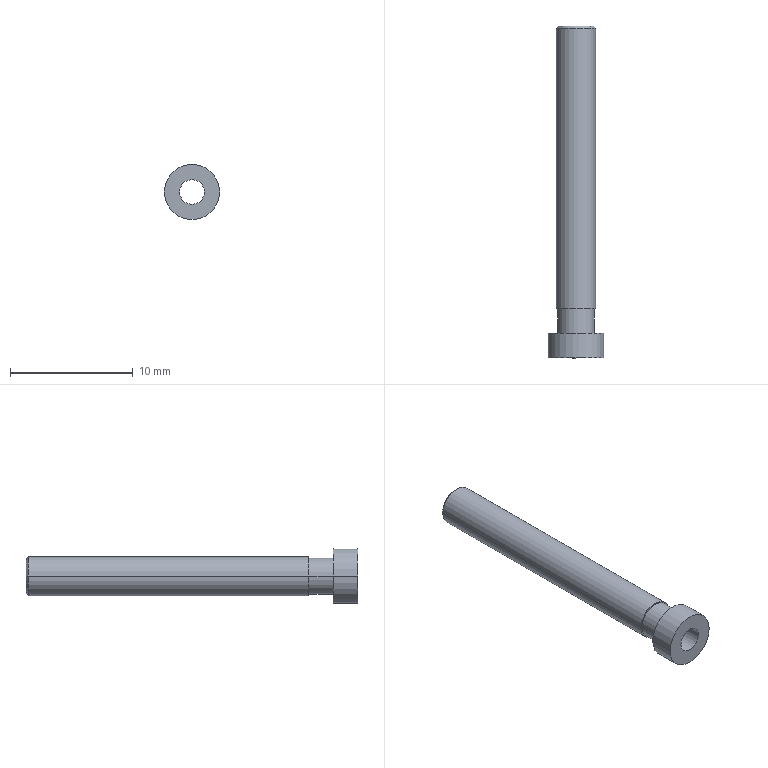Part | STEP file | BU-A08 | 1 solid | 14 faces | box 4.5 x 27 x 4.5 mm | volume 144.202 mm3 | cylinder 8 | plane 4 | cone 2 | commonest cylinder face diameters 2.02 x2 3 x2 3.2 x2 4.5 x2
STEP:
#1=CARTESIAN_POINT('',(0.,0.,0.));
#2=DIRECTION('',(0.,0.,1.));
#3=DIRECTION('',(1.,0.,0.));
#4=AXIS2_PLACEMENT_3D('',#1,#2,#3);
#5=CARTESIAN_POINT('',(-1.4,27.,0.));
#6=VERTEX_POINT('',#5);
#7=CARTESIAN_POINT('',(1.4,27.,0.));
#8=VERTEX_POINT('',#7);
#9=CARTESIAN_POINT('',(0.,27.,0.));
#10=DIRECTION('',(0.,1.,0.));
#11=DIRECTION('',(-1.,0.,0.));
#12=AXIS2_PLACEMENT_3D('',#9,#10,#11);
#13=CIRCLE('',#12,1.4);
#14=CARTESIAN_POINT('',(0.,26.8,0.));
#15=DIRECTION('',(0.,-1.,0.));
#16=DIRECTION('',(1.,0.,0.));
#17=AXIS2_PLACEMENT_3D('',#14,#15,#16);
#18=CONICAL_SURFACE('',#17,1.6,0.7854);
#19=CARTESIAN_POINT('',(3.142,-0.2));
#20=DIRECTION('',(-1.,0.));
#21=VECTOR('',#20,1.);
#22=LINE('',#19,#21);
#23=(GEOMETRIC_REPRESENTATION_CONTEXT(2)PARAMETRIC_REPRESENTATION_CONTEXT()REPRESENTATION_CONTEXT('',''));
#24=DEFINITIONAL_REPRESENTATION('',(#22),#23);
#25=PCURVE('',#18,#24);
#26=CARTESIAN_POINT('',(1.6,27.,0.));
#27=DIRECTION('',(0.,1.,0.));
#28=DIRECTION('',(-1.,0.,0.));
#29=AXIS2_PLACEMENT_3D('',#26,#27,#28);
#30=PLANE('',#29);
#31=CARTESIAN_POINT('',(1.6,0.));
#32=DIRECTION('',(1.,0.));
#33=AXIS2_PLACEMENT_2D('',#31,#32);
#34=CIRCLE('',#33,1.4);
#35=(GEOMETRIC_REPRESENTATION_CONTEXT(2)PARAMETRIC_REPRESENTATION_CONTEXT()REPRESENTATION_CONTEXT('',''));
#36=DEFINITIONAL_REPRESENTATION('',(#34),#35);
#37=PCURVE('',#30,#36);
#38=SURFACE_CURVE('',#13,(#25,#37),.PCURVE_S1.);
#39=EDGE_CURVE('',#6,#8,#38,.T.);
#40=ORIENTED_EDGE('',*,*,#39,.F.);
#41=CARTESIAN_POINT('',(-1.6,26.8,0.));
#42=VERTEX_POINT('',#41);
#43=CARTESIAN_POINT('',(-1.6,26.8,0.));
#44=DIRECTION('',(-0.7071,-0.7071,0.));
#45=VECTOR('',#44,1.);
#46=LINE('',#43,#45);
#47=CARTESIAN_POINT('',(3.142,0.));
#48=DIRECTION('',(0.,1.));
#49=VECTOR('',#48,1.);
#50=LINE('',#47,#49);
#51=(GEOMETRIC_REPRESENTATION_CONTEXT(2)PARAMETRIC_REPRESENTATION_CONTEXT()REPRESENTATION_CONTEXT('',''));
#52=DEFINITIONAL_REPRESENTATION('',(#50),#51);
#53=PCURVE('',#18,#52);
#54=CARTESIAN_POINT('',(0.,26.8,0.));
#55=DIRECTION('',(0.,-1.,0.));
#56=DIRECTION('',(1.,0.,0.));
#57=AXIS2_PLACEMENT_3D('',#54,#55,#56);
#58=CONICAL_SURFACE('',#57,1.6,0.7854);
#59=CARTESIAN_POINT('',(3.142,0.));
#60=DIRECTION('',(0.,1.));
#61=VECTOR('',#60,1.);
#62=LINE('',#59,#61);
#63=(GEOMETRIC_REPRESENTATION_CONTEXT(2)PARAMETRIC_REPRESENTATION_CONTEXT()REPRESENTATION_CONTEXT('',''));
#64=DEFINITIONAL_REPRESENTATION('',(#62),#63);
#65=PCURVE('',#58,#64);
#66=SURFACE_CURVE('',#46,(#53,#65),.PCURVE_S1.);
#67=EDGE_CURVE('',#6,#42,#66,.T.);
#68=ORIENTED_EDGE('',*,*,#67,.T.);
#69=CARTESIAN_POINT('',(1.6,26.8,0.));
#70=VERTEX_POINT('',#69);
#71=CARTESIAN_POINT('',(0.,26.8,0.));
#72=DIRECTION('',(0.,-1.,0.));
#73=DIRECTION('',(-1.,0.,0.));
#74=AXIS2_PLACEMENT_3D('',#71,#72,#73);
#75=CIRCLE('',#74,1.6);
#76=CARTESIAN_POINT('',(-3.142,0.));
#77=DIRECTION('',(1.,0.));
#78=VECTOR('',#77,1.);
#79=LINE('',#76,#78);
#80=(GEOMETRIC_REPRESENTATION_CONTEXT(2)PARAMETRIC_REPRESENTATION_CONTEXT()REPRESENTATION_CONTEXT('',''));
#81=DEFINITIONAL_REPRESENTATION('',(#79),#80);
#82=PCURVE('',#18,#81);
#83=CARTESIAN_POINT('',(0.,-1000.,0.));
#84=DIRECTION('',(0.,-1.,0.));
#85=DIRECTION('',(1.,0.,0.));
#86=AXIS2_PLACEMENT_3D('',#83,#84,#85);
#87=CYLINDRICAL_SURFACE('',#86,1.6);
#88=CARTESIAN_POINT('',(-3.142,-1026.8));
#89=DIRECTION('',(1.,0.));
#90=VECTOR('',#89,1.);
#91=LINE('',#88,#90);
#92=(GEOMETRIC_REPRESENTATION_CONTEXT(2)PARAMETRIC_REPRESENTATION_CONTEXT()REPRESENTATION_CONTEXT('',''));
#93=DEFINITIONAL_REPRESENTATION('',(#91),#92);
#94=PCURVE('',#87,#93);
#95=SURFACE_CURVE('',#75,(#82,#94),.PCURVE_S1.);
#96=EDGE_CURVE('',#70,#42,#95,.T.);
#97=ORIENTED_EDGE('',*,*,#96,.F.);
#98=CARTESIAN_POINT('',(1.6,26.8,0.));
#99=DIRECTION('',(0.7071,-0.7071,0.));
#100=VECTOR('',#99,1.);
#101=LINE('',#98,#100);
#102=CARTESIAN_POINT('',(0.,0.));
#103=DIRECTION('',(0.,1.));
#104=VECTOR('',#103,1.);
#105=LINE('',#102,#104);
#106=(GEOMETRIC_REPRESENTATION_CONTEXT(2)PARAMETRIC_REPRESENTATION_CONTEXT()REPRESENTATION_CONTEXT('',''));
#107=DEFINITIONAL_REPRESENTATION('',(#105),#106);
#108=PCURVE('',#18,#107);
#109=CARTESIAN_POINT('',(6.283,0.));
#110=DIRECTION('',(0.,1.));
#111=VECTOR('',#110,1.);
#112=LINE('',#109,#111);
#113=(GEOMETRIC_REPRESENTATION_CONTEXT(2)PARAMETRIC_REPRESENTATION_CONTEXT()REPRESENTATION_CONTEXT('',''));
#114=DEFINITIONAL_REPRESENTATION('',(#112),#113);
#115=PCURVE('',#58,#114);
#116=SURFACE_CURVE('',#101,(#108,#115),.PCURVE_S1.);
#117=EDGE_CURVE('',#8,#70,#116,.T.);
#118=ORIENTED_EDGE('',*,*,#117,.F.);
#119=EDGE_LOOP('',(#40,#68,#97,#118));
#120=FACE_BOUND('',#119,.T.);
#121=ADVANCED_FACE('',(#120),#18,.T.);
#122=CARTESIAN_POINT('',(1.01,27.,0.));
#123=VERTEX_POINT('',#122);
#124=CARTESIAN_POINT('',(1.01,0.,0.));
#125=VERTEX_POINT('',#124);
#126=CARTESIAN_POINT('',(1.01,-1000.,0.));
#127=DIRECTION('',(0.,-1.,0.));
#128=VECTOR('',#127,1.);
#129=LINE('',#126,#128);
#130=CARTESIAN_POINT('',(0.,-1000.,0.));
#131=DIRECTION('',(0.,-1.,0.));
#132=DIRECTION('',(1.,0.,0.));
#133=AXIS2_PLACEMENT_3D('',#130,#131,#132);
#134=CYLINDRICAL_SURFACE('',#133,1.01);
#135=CARTESIAN_POINT('',(6.283,0.));
#136=DIRECTION('',(0.,1.));
#137=VECTOR('',#136,1.);
#138=LINE('',#135,#137);
#139=(GEOMETRIC_REPRESENTATION_CONTEXT(2)PARAMETRIC_REPRESENTATION_CONTEXT()REPRESENTATION_CONTEXT('',''));
#140=DEFINITIONAL_REPRESENTATION('',(#138),#139);
#141=PCURVE('',#134,#140);
#142=CARTESIAN_POINT('',(0.,-1000.,0.));
#143=DIRECTION('',(0.,-1.,0.));
#144=DIRECTION('',(1.,0.,0.));
#145=AXIS2_PLACEMENT_3D('',#142,#143,#144);
#146=CYLINDRICAL_SURFACE('',#145,1.01);
#147=CARTESIAN_POINT('',(0.,0.));
#148=DIRECTION('',(0.,1.));
#149=VECTOR('',#148,1.);
#150=LINE('',#147,#149);
#151=(GEOMETRIC_REPRESENTATION_CONTEXT(2)PARAMETRIC_REPRESENTATION_CONTEXT()REPRESENTATION_CONTEXT('',''));
#152=DEFINITIONAL_REPRESENTATION('',(#150),#151);
#153=PCURVE('',#146,#152);
#154=SURFACE_CURVE('',#129,(#141,#153),.PCURVE_S1.);
#155=EDGE_CURVE('',#123,#125,#154,.T.);
#156=ORIENTED_EDGE('',*,*,#155,.T.);
#157=CARTESIAN_POINT('',(-1.01,0.,0.));
#158=VERTEX_POINT('',#157);
#159=CARTESIAN_POINT('',(0.,0.,0.));
#160=DIRECTION('',(0.,-1.,0.));
#161=DIRECTION('',(1.,0.,0.));
#162=AXIS2_PLACEMENT_3D('',#159,#160,#161);
#163=CIRCLE('',#162,1.01);
#164=CARTESIAN_POINT('',(0.,-1000.));
#165=DIRECTION('',(1.,0.));
#166=VECTOR('',#165,1.);
#167=LINE('',#164,#166);
#168=(GEOMETRIC_REPRESENTATION_CONTEXT(2)PARAMETRIC_REPRESENTATION_CONTEXT()REPRESENTATION_CONTEXT('',''));
#169=DEFINITIONAL_REPRESENTATION('',(#167),#168);
#170=PCURVE('',#134,#169);
#171=CARTESIAN_POINT('',(1.01,0.,0.));
#172=DIRECTION('',(0.,-1.,0.));
#173=DIRECTION('',(1.,0.,0.));
#174=AXIS2_PLACEMENT_3D('',#171,#172,#173);
#175=PLANE('',#174);
#176=CARTESIAN_POINT('',(-1.01,0.));
#177=DIRECTION('',(1.,0.));
#178=AXIS2_PLACEMENT_2D('',#176,#177);
#179=CIRCLE('',#178,1.01);
#180=(GEOMETRIC_REPRESENTATION_CONTEXT(2)PARAMETRIC_REPRESENTATION_CONTEXT()REPRESENTATION_CONTEXT('',''));
#181=DEFINITIONAL_REPRESENTATION('',(#179),#180);
#182=PCURVE('',#175,#181);
#183=SURFACE_CURVE('',#163,(#170,#182),.PCURVE_S1.);
#184=EDGE_CURVE('',#158,#125,#183,.T.);
#185=ORIENTED_EDGE('',*,*,#184,.F.);
#186=CARTESIAN_POINT('',(-1.01,27.,0.));
#187=VERTEX_POINT('',#186);
#188=CARTESIAN_POINT('',(-1.01,-1000.,0.));
#189=DIRECTION('',(0.,-1.,0.));
#190=VECTOR('',#189,1.);
#191=LINE('',#188,#190);
#192=CARTESIAN_POINT('',(3.142,0.));
#193=DIRECTION('',(0.,1.));
#194=VECTOR('',#193,1.);
#195=LINE('',#192,#194);
#196=(GEOMETRIC_REPRESENTATION_CONTEXT(2)PARAMETRIC_REPRESENTATION_CONTEXT()REPRESENTATION_CONTEXT('',''));
#197=DEFINITIONAL_REPRESENTATION('',(#195),#196);
#198=PCURVE('',#134,#197);
#199=CARTESIAN_POINT('',(3.142,0.));
#200=DIRECTION('',(0.,1.));
#201=VECTOR('',#200,1.);
#202=LINE('',#199,#201);
#203=(GEOMETRIC_REPRESENTATION_CONTEXT(2)PARAMETRIC_REPRESENTATION_CONTEXT()REPRESENTATION_CONTEXT('',''));
#204=DEFINITIONAL_REPRESENTATION('',(#202),#203);
#205=PCURVE('',#146,#204);
#206=SURFACE_CURVE('',#191,(#198,#205),.PCURVE_S1.);
#207=EDGE_CURVE('',#187,#158,#206,.T.);
#208=ORIENTED_EDGE('',*,*,#207,.F.);
#209=CARTESIAN_POINT('',(0.,27.,0.));
#210=DIRECTION('',(0.,-1.,0.));
#211=DIRECTION('',(1.,0.,0.));
#212=AXIS2_PLACEMENT_3D('',#209,#210,#211);
#213=CIRCLE('',#212,1.01);
#214=CARTESIAN_POINT('',(0.,-1027.));
#215=DIRECTION('',(1.,0.));
#216=VECTOR('',#215,1.);
#217=LINE('',#214,#216);
#218=(GEOMETRIC_REPRESENTATION_CONTEXT(2)PARAMETRIC_REPRESENTATION_CONTEXT()REPRESENTATION_CONTEXT('',''));
#219=DEFINITIONAL_REPRESENTATION('',(#217),#218);
#220=PCURVE('',#134,#219);
#221=CARTESIAN_POINT('',(0.59,0.));
#222=CARTESIAN_POINT('',(0.59,1.749));
#223=CARTESIAN_POINT('',(2.105,0.8747));
#224=CARTESIAN_POINT('',(3.62,0.));
#225=CARTESIAN_POINT('',(2.105,-0.8747));
#226=CARTESIAN_POINT('',(0.59,-1.749));
#227=CARTESIAN_POINT('',(0.59,0.));
#228=(BOUNDED_CURVE()B_SPLINE_CURVE(2,(#221,#222,#223,#224,#225,#226,#227),.UNSPECIFIED.,.T.,.F.)B_SPLINE_CURVE_WITH_KNOTS((1,2,2,2,2,1),(-2.094,0.,2.094,4.189,6.283,8.378),.UNSPECIFIED.)CURVE()GEOMETRIC_REPRESENTATION_ITEM()RATIONAL_B_SPLINE_CURVE((1.,0.5,1.,0.5,1.,0.5,1.))REPRESENTATION_ITEM(''));
#229=(GEOMETRIC_REPRESENTATION_CONTEXT(2)PARAMETRIC_REPRESENTATION_CONTEXT()REPRESENTATION_CONTEXT('',''));
#230=DEFINITIONAL_REPRESENTATION('',(#228),#229);
#231=PCURVE('',#30,#230);
#232=SURFACE_CURVE('',#213,(#220,#231),.PCURVE_S1.);
#233=EDGE_CURVE('',#187,#123,#232,.T.);
#234=ORIENTED_EDGE('',*,*,#233,.T.);
#235=EDGE_LOOP('',(#156,#185,#208,#234));
#236=FACE_BOUND('',#235,.F.);
#237=ADVANCED_FACE('',(#236),#134,.F.);
#238=ORIENTED_EDGE('',*,*,#96,.T.);
#239=CARTESIAN_POINT('',(-1.6,4.,0.));
#240=VERTEX_POINT('',#239);
#241=CARTESIAN_POINT('',(-1.6,-1000.,0.));
#242=DIRECTION('',(0.,-1.,0.));
#243=VECTOR('',#242,1.);
#244=LINE('',#241,#243);
#245=CARTESIAN_POINT('',(3.142,0.));
#246=DIRECTION('',(0.,1.));
#247=VECTOR('',#246,1.);
#248=LINE('',#245,#247);
#249=(GEOMETRIC_REPRESENTATION_CONTEXT(2)PARAMETRIC_REPRESENTATION_CONTEXT()REPRESENTATION_CONTEXT('',''));
#250=DEFINITIONAL_REPRESENTATION('',(#248),#249);
#251=PCURVE('',#87,#250);
#252=CARTESIAN_POINT('',(0.,-1000.,0.));
#253=DIRECTION('',(0.,-1.,0.));
#254=DIRECTION('',(1.,0.,0.));
#255=AXIS2_PLACEMENT_3D('',#252,#253,#254);
#256=CYLINDRICAL_SURFACE('',#255,1.6);
#257=CARTESIAN_POINT('',(3.142,0.));
#258=DIRECTION('',(0.,1.));
#259=VECTOR('',#258,1.);
#260=LINE('',#257,#259);
#261=(GEOMETRIC_REPRESENTATION_CONTEXT(2)PARAMETRIC_REPRESENTATION_CONTEXT()REPRESENTATION_CONTEXT('',''));
#262=DEFINITIONAL_REPRESENTATION('',(#260),#261);
#263=PCURVE('',#256,#262);
#264=SURFACE_CURVE('',#244,(#251,#263),.PCURVE_S1.);
#265=EDGE_CURVE('',#42,#240,#264,.T.);
#266=ORIENTED_EDGE('',*,*,#265,.T.);
#267=CARTESIAN_POINT('',(1.6,4.,0.));
#268=VERTEX_POINT('',#267);
#269=CARTESIAN_POINT('',(0.,4.,0.));
#270=DIRECTION('',(0.,-1.,0.));
#271=DIRECTION('',(1.,0.,0.));
#272=AXIS2_PLACEMENT_3D('',#269,#270,#271);
#273=CIRCLE('',#272,1.6);
#274=CARTESIAN_POINT('',(0.,-1004.));
#275=DIRECTION('',(1.,0.));
#276=VECTOR('',#275,1.);
#277=LINE('',#274,#276);
#278=(GEOMETRIC_REPRESENTATION_CONTEXT(2)PARAMETRIC_REPRESENTATION_CONTEXT()REPRESENTATION_CONTEXT('',''));
#279=DEFINITIONAL_REPRESENTATION('',(#277),#278);
#280=PCURVE('',#87,#279);
#281=CARTESIAN_POINT('',(1.5,4.,0.));
#282=DIRECTION('',(0.,-1.,0.));
#283=DIRECTION('',(1.,0.,0.));
#284=AXIS2_PLACEMENT_3D('',#281,#282,#283);
#285=PLANE('',#284);
#286=CARTESIAN_POINT('',(-1.5,0.));
#287=DIRECTION('',(1.,0.));
#288=AXIS2_PLACEMENT_2D('',#286,#287);
#289=CIRCLE('',#288,1.6);
#290=(GEOMETRIC_REPRESENTATION_CONTEXT(2)PARAMETRIC_REPRESENTATION_CONTEXT()REPRESENTATION_CONTEXT('',''));
#291=DEFINITIONAL_REPRESENTATION('',(#289),#290);
#292=PCURVE('',#285,#291);
#293=SURFACE_CURVE('',#273,(#280,#292),.PCURVE_S1.);
#294=EDGE_CURVE('',#268,#240,#293,.T.);
#295=ORIENTED_EDGE('',*,*,#294,.F.);
#296=CARTESIAN_POINT('',(1.6,-1000.,0.));
#297=DIRECTION('',(0.,-1.,0.));
#298=VECTOR('',#297,1.);
#299=LINE('',#296,#298);
#300=CARTESIAN_POINT('',(0.,0.));
#301=DIRECTION('',(0.,1.));
#302=VECTOR('',#301,1.);
#303=LINE('',#300,#302);
#304=(GEOMETRIC_REPRESENTATION_CONTEXT(2)PARAMETRIC_REPRESENTATION_CONTEXT()REPRESENTATION_CONTEXT('',''));
#305=DEFINITIONAL_REPRESENTATION('',(#303),#304);
#306=PCURVE('',#87,#305);
#307=CARTESIAN_POINT('',(6.283,0.));
#308=DIRECTION('',(0.,1.));
#309=VECTOR('',#308,1.);
#310=LINE('',#307,#309);
#311=(GEOMETRIC_REPRESENTATION_CONTEXT(2)PARAMETRIC_REPRESENTATION_CONTEXT()REPRESENTATION_CONTEXT('',''));
#312=DEFINITIONAL_REPRESENTATION('',(#310),#311);
#313=PCURVE('',#256,#312);
#314=SURFACE_CURVE('',#299,(#306,#313),.PCURVE_S1.);
#315=EDGE_CURVE('',#70,#268,#314,.T.);
#316=ORIENTED_EDGE('',*,*,#315,.F.);
#317=EDGE_LOOP('',(#238,#266,#295,#316));
#318=FACE_BOUND('',#317,.T.);
#319=ADVANCED_FACE('',(#318),#87,.T.);
#320=CARTESIAN_POINT('',(1.5,4.,0.));
#321=VERTEX_POINT('',#320);
#322=CARTESIAN_POINT('',(-1.5,4.,0.));
#323=VERTEX_POINT('',#322);
#324=CARTESIAN_POINT('',(0.,4.,0.));
#325=DIRECTION('',(0.,-1.,0.));
#326=DIRECTION('',(1.,0.,0.));
#327=AXIS2_PLACEMENT_3D('',#324,#325,#326);
#328=CIRCLE('',#327,1.5);
#329=CARTESIAN_POINT('',(0.,-1000.,0.));
#330=DIRECTION('',(0.,-1.,0.));
#331=DIRECTION('',(1.,0.,0.));
#332=AXIS2_PLACEMENT_3D('',#329,#330,#331);
#333=CYLINDRICAL_SURFACE('',#332,1.5);
#334=CARTESIAN_POINT('',(0.,-1004.));
#335=DIRECTION('',(1.,0.));
#336=VECTOR('',#335,1.);
#337=LINE('',#334,#336);
#338=(GEOMETRIC_REPRESENTATION_CONTEXT(2)PARAMETRIC_REPRESENTATION_CONTEXT()REPRESENTATION_CONTEXT('',''));
#339=DEFINITIONAL_REPRESENTATION('',(#337),#338);
#340=PCURVE('',#333,#339);
#341=CARTESIAN_POINT('',(-1.5,0.));
#342=DIRECTION('',(1.,0.));
#343=AXIS2_PLACEMENT_2D('',#341,#342);
#344=CIRCLE('',#343,1.5);
#345=(GEOMETRIC_REPRESENTATION_CONTEXT(2)PARAMETRIC_REPRESENTATION_CONTEXT()REPRESENTATION_CONTEXT('',''));
#346=DEFINITIONAL_REPRESENTATION('',(#344),#345);
#347=PCURVE('',#285,#346);
#348=SURFACE_CURVE('',#328,(#340,#347),.PCURVE_S1.);
#349=EDGE_CURVE('',#321,#323,#348,.T.);
#350=ORIENTED_EDGE('',*,*,#349,.T.);
#351=CARTESIAN_POINT('',(-1.5,2.,0.));
#352=VERTEX_POINT('',#351);
#353=CARTESIAN_POINT('',(-1.5,-1000.,0.));
#354=DIRECTION('',(0.,-1.,0.));
#355=VECTOR('',#354,1.);
#356=LINE('',#353,#355);
#357=CARTESIAN_POINT('',(3.142,0.));
#358=DIRECTION('',(0.,1.));
#359=VECTOR('',#358,1.);
#360=LINE('',#357,#359);
#361=(GEOMETRIC_REPRESENTATION_CONTEXT(2)PARAMETRIC_REPRESENTATION_CONTEXT()REPRESENTATION_CONTEXT('',''));
#362=DEFINITIONAL_REPRESENTATION('',(#360),#361);
#363=PCURVE('',#333,#362);
#364=CARTESIAN_POINT('',(0.,-1000.,0.));
#365=DIRECTION('',(0.,-1.,0.));
#366=DIRECTION('',(1.,0.,0.));
#367=AXIS2_PLACEMENT_3D('',#364,#365,#366);
#368=CYLINDRICAL_SURFACE('',#367,1.5);
#369=CARTESIAN_POINT('',(3.142,0.));
#370=DIRECTION('',(0.,1.));
#371=VECTOR('',#370,1.);
#372=LINE('',#369,#371);
#373=(GEOMETRIC_REPRESENTATION_CONTEXT(2)PARAMETRIC_REPRESENTATION_CONTEXT()REPRESENTATION_CONTEXT('',''));
#374=DEFINITIONAL_REPRESENTATION('',(#372),#373);
#375=PCURVE('',#368,#374);
#376=SURFACE_CURVE('',#356,(#363,#375),.PCURVE_S1.);
#377=EDGE_CURVE('',#323,#352,#376,.T.);
#378=ORIENTED_EDGE('',*,*,#377,.T.);
#379=CARTESIAN_POINT('',(1.5,2.,0.));
#380=VERTEX_POINT('',#379);
#381=CARTESIAN_POINT('',(0.,2.,0.));
#382=DIRECTION('',(0.,-1.,0.));
#383=DIRECTION('',(1.,0.,0.));
#384=AXIS2_PLACEMENT_3D('',#381,#382,#383);
#385=CIRCLE('',#384,1.5);
#386=CARTESIAN_POINT('',(0.,-1002.));
#387=DIRECTION('',(1.,0.));
#388=VECTOR('',#387,1.);
#389=LINE('',#386,#388);
#390=(GEOMETRIC_REPRESENTATION_CONTEXT(2)PARAMETRIC_REPRESENTATION_CONTEXT()REPRESENTATION_CONTEXT('',''));
#391=DEFINITIONAL_REPRESENTATION('',(#389),#390);
#392=PCURVE('',#333,#391);
#393=CARTESIAN_POINT('',(2.25,2.,0.));
#394=DIRECTION('',(0.,1.,0.));
#395=DIRECTION('',(-1.,0.,0.));
#396=AXIS2_PLACEMENT_3D('',#393,#394,#395);
#397=PLANE('',#396);
#398=CARTESIAN_POINT('',(0.75,0.));
#399=CARTESIAN_POINT('',(0.75,2.598));
#400=CARTESIAN_POINT('',(3.,1.299));
#401=CARTESIAN_POINT('',(5.25,0.));
#402=CARTESIAN_POINT('',(3.,-1.299));
#403=CARTESIAN_POINT('',(0.75,-2.598));
#404=CARTESIAN_POINT('',(0.75,0.));
#405=(BOUNDED_CURVE()B_SPLINE_CURVE(2,(#398,#399,#400,#401,#402,#403,#404),.UNSPECIFIED.,.T.,.F.)B_SPLINE_CURVE_WITH_KNOTS((1,2,2,2,2,1),(-2.094,0.,2.094,4.189,6.283,8.378),.UNSPECIFIED.)CURVE()GEOMETRIC_REPRESENTATION_ITEM()RATIONAL_B_SPLINE_CURVE((1.,0.5,1.,0.5,1.,0.5,1.))REPRESENTATION_ITEM(''));
#406=(GEOMETRIC_REPRESENTATION_CONTEXT(2)PARAMETRIC_REPRESENTATION_CONTEXT()REPRESENTATION_CONTEXT('',''));
#407=DEFINITIONAL_REPRESENTATION('',(#405),#406);
#408=PCURVE('',#397,#407);
#409=SURFACE_CURVE('',#385,(#392,#408),.PCURVE_S1.);
#410=EDGE_CURVE('',#380,#352,#409,.T.);
#411=ORIENTED_EDGE('',*,*,#410,.F.);
#412=CARTESIAN_POINT('',(1.5,-1000.,0.));
#413=DIRECTION('',(0.,-1.,0.));
#414=VECTOR('',#413,1.);
#415=LINE('',#412,#414);
#416=CARTESIAN_POINT('',(0.,0.));
#417=DIRECTION('',(0.,1.));
#418=VECTOR('',#417,1.);
#419=LINE('',#416,#418);
#420=(GEOMETRIC_REPRESENTATION_CONTEXT(2)PARAMETRIC_REPRESENTATION_CONTEXT()REPRESENTATION_CONTEXT('',''));
#421=DEFINITIONAL_REPRESENTATION('',(#419),#420);
#422=PCURVE('',#333,#421);
#423=CARTESIAN_POINT('',(6.283,0.));
#424=DIRECTION('',(0.,1.));
#425=VECTOR('',#424,1.);
#426=LINE('',#423,#425);
#427=(GEOMETRIC_REPRESENTATION_CONTEXT(2)PARAMETRIC_REPRESENTATION_CONTEXT()REPRESENTATION_CONTEXT('',''));
#428=DEFINITIONAL_REPRESENTATION('',(#426),#427);
#429=PCURVE('',#368,#428);
#430=SURFACE_CURVE('',#415,(#422,#429),.PCURVE_S1.);
#431=EDGE_CURVE('',#321,#380,#430,.T.);
#432=ORIENTED_EDGE('',*,*,#431,.F.);
#433=EDGE_LOOP('',(#350,#378,#411,#432));
#434=FACE_BOUND('',#433,.T.);
#435=ADVANCED_FACE('',(#434),#333,.T.);
#436=CARTESIAN_POINT('',(2.25,2.,0.));
#437=VERTEX_POINT('',#436);
#438=CARTESIAN_POINT('',(-2.25,2.,0.));
#439=VERTEX_POINT('',#438);
#440=CARTESIAN_POINT('',(0.,2.,0.));
#441=DIRECTION('',(0.,-1.,0.));
#442=DIRECTION('',(1.,0.,0.));
#443=AXIS2_PLACEMENT_3D('',#440,#441,#442);
#444=CIRCLE('',#443,2.25);
#445=CARTESIAN_POINT('',(0.,-1000.,0.));
#446=DIRECTION('',(0.,-1.,0.));
#447=DIRECTION('',(1.,0.,0.));
#448=AXIS2_PLACEMENT_3D('',#445,#446,#447);
#449=CYLINDRICAL_SURFACE('',#448,2.25);
#450=CARTESIAN_POINT('',(0.,-1002.));
#451=DIRECTION('',(1.,0.));
#452=VECTOR('',#451,1.);
#453=LINE('',#450,#452);
#454=(GEOMETRIC_REPRESENTATION_CONTEXT(2)PARAMETRIC_REPRESENTATION_CONTEXT()REPRESENTATION_CONTEXT('',''));
#455=DEFINITIONAL_REPRESENTATION('',(#453),#454);
#456=PCURVE('',#449,#455);
#457=CARTESIAN_POINT('',(0.,0.));
#458=CARTESIAN_POINT('',(0.,3.897));
#459=CARTESIAN_POINT('',(3.375,1.949));
#460=CARTESIAN_POINT('',(6.75,0.));
#461=CARTESIAN_POINT('',(3.375,-1.949));
#462=CARTESIAN_POINT('',(0.,-3.897));
#463=CARTESIAN_POINT('',(0.,0.));
#464=(BOUNDED_CURVE()B_SPLINE_CURVE(2,(#457,#458,#459,#460,#461,#462,#463),.UNSPECIFIED.,.T.,.F.)B_SPLINE_CURVE_WITH_KNOTS((1,2,2,2,2,1),(-2.094,0.,2.094,4.189,6.283,8.378),.UNSPECIFIED.)CURVE()GEOMETRIC_REPRESENTATION_ITEM()RATIONAL_B_SPLINE_CURVE((1.,0.5,1.,0.5,1.,0.5,1.))REPRESENTATION_ITEM(''));
#465=(GEOMETRIC_REPRESENTATION_CONTEXT(2)PARAMETRIC_REPRESENTATION_CONTEXT()REPRESENTATION_CONTEXT('',''));
#466=DEFINITIONAL_REPRESENTATION('',(#464),#465);
#467=PCURVE('',#397,#466);
#468=SURFACE_CURVE('',#444,(#456,#467),.PCURVE_S1.);
#469=EDGE_CURVE('',#437,#439,#468,.T.);
#470=ORIENTED_EDGE('',*,*,#469,.T.);
#471=CARTESIAN_POINT('',(-2.25,0.,0.));
#472=VERTEX_POINT('',#471);
#473=CARTESIAN_POINT('',(-2.25,-1000.,0.));
#474=DIRECTION('',(0.,-1.,0.));
#475=VECTOR('',#474,1.);
#476=LINE('',#473,#475);
#477=CARTESIAN_POINT('',(3.142,0.));
#478=DIRECTION('',(0.,1.));
#479=VECTOR('',#478,1.);
#480=LINE('',#477,#479);
#481=(GEOMETRIC_REPRESENTATION_CONTEXT(2)PARAMETRIC_REPRESENTATION_CONTEXT()REPRESENTATION_CONTEXT('',''));
#482=DEFINITIONAL_REPRESENTATION('',(#480),#481);
#483=PCURVE('',#449,#482);
#484=CARTESIAN_POINT('',(0.,-1000.,0.));
#485=DIRECTION('',(0.,-1.,0.));
#486=DIRECTION('',(1.,0.,0.));
#487=AXIS2_PLACEMENT_3D('',#484,#485,#486);
#488=CYLINDRICAL_SURFACE('',#487,2.25);
#489=CARTESIAN_POINT('',(3.142,0.));
#490=DIRECTION('',(0.,1.));
#491=VECTOR('',#490,1.);
#492=LINE('',#489,#491);
#493=(GEOMETRIC_REPRESENTATION_CONTEXT(2)PARAMETRIC_REPRESENTATION_CONTEXT()REPRESENTATION_CONTEXT('',''));
#494=DEFINITIONAL_REPRESENTATION('',(#492),#493);
#495=PCURVE('',#488,#494);
#496=SURFACE_CURVE('',#476,(#483,#495),.PCURVE_S1.);
#497=EDGE_CURVE('',#439,#472,#496,.T.);
#498=ORIENTED_EDGE('',*,*,#497,.T.);
#499=CARTESIAN_POINT('',(2.25,0.,0.));
#500=VERTEX_POINT('',#499);
#501=CARTESIAN_POINT('',(0.,0.,0.));
#502=DIRECTION('',(0.,-1.,0.));
#503=DIRECTION('',(1.,0.,0.));
#504=AXIS2_PLACEMENT_3D('',#501,#502,#503);
#505=CIRCLE('',#504,2.25);
#506=CARTESIAN_POINT('',(0.,-1000.));
#507=DIRECTION('',(1.,0.));
#508=VECTOR('',#507,1.);
#509=LINE('',#506,#508);
#510=(GEOMETRIC_REPRESENTATION_CONTEXT(2)PARAMETRIC_REPRESENTATION_CONTEXT()REPRESENTATION_CONTEXT('',''));
#511=DEFINITIONAL_REPRESENTATION('',(#509),#510);
#512=PCURVE('',#449,#511);
#513=CARTESIAN_POINT('',(-1.01,0.));
#514=DIRECTION('',(1.,0.));
#515=AXIS2_PLACEMENT_2D('',#513,#514);
#516=CIRCLE('',#515,2.25);
#517=(GEOMETRIC_REPRESENTATION_CONTEXT(2)PARAMETRIC_REPRESENTATION_CONTEXT()REPRESENTATION_CONTEXT('',''));
#518=DEFINITIONAL_REPRESENTATION('',(#516),#517);
#519=PCURVE('',#175,#518);
#520=SURFACE_CURVE('',#505,(#512,#519),.PCURVE_S1.);
#521=EDGE_CURVE('',#500,#472,#520,.T.);
#522=ORIENTED_EDGE('',*,*,#521,.F.);
#523=CARTESIAN_POINT('',(2.25,-1000.,0.));
#524=DIRECTION('',(0.,-1.,0.));
#525=VECTOR('',#524,1.);
#526=LINE('',#523,#525);
#527=CARTESIAN_POINT('',(0.,0.));
#528=DIRECTION('',(0.,1.));
#529=VECTOR('',#528,1.);
#530=LINE('',#527,#529);
#531=(GEOMETRIC_REPRESENTATION_CONTEXT(2)PARAMETRIC_REPRESENTATION_CONTEXT()REPRESENTATION_CONTEXT('',''));
#532=DEFINITIONAL_REPRESENTATION('',(#530),#531);
#533=PCURVE('',#449,#532);
#534=CARTESIAN_POINT('',(6.283,0.));
#535=DIRECTION('',(0.,1.));
#536=VECTOR('',#535,1.);
#537=LINE('',#534,#536);
#538=(GEOMETRIC_REPRESENTATION_CONTEXT(2)PARAMETRIC_REPRESENTATION_CONTEXT()REPRESENTATION_CONTEXT('',''));
#539=DEFINITIONAL_REPRESENTATION('',(#537),#538);
#540=PCURVE('',#488,#539);
#541=SURFACE_CURVE('',#526,(#533,#540),.PCURVE_S1.);
#542=EDGE_CURVE('',#437,#500,#541,.T.);
#543=ORIENTED_EDGE('',*,*,#542,.F.);
#544=EDGE_LOOP('',(#470,#498,#522,#543));
#545=FACE_BOUND('',#544,.T.);
#546=ADVANCED_FACE('',(#545),#449,.T.);
#547=ORIENTED_EDGE('',*,*,#497,.F.);
#548=CARTESIAN_POINT('',(0.,2.,0.));
#549=DIRECTION('',(0.,-1.,0.));
#550=DIRECTION('',(1.,0.,0.));
#551=AXIS2_PLACEMENT_3D('',#548,#549,#550);
#552=CIRCLE('',#551,2.25);
#553=CARTESIAN_POINT('',(0.,-1002.));
#554=DIRECTION('',(1.,0.));
#555=VECTOR('',#554,1.);
#556=LINE('',#553,#555);
#557=(GEOMETRIC_REPRESENTATION_CONTEXT(2)PARAMETRIC_REPRESENTATION_CONTEXT()REPRESENTATION_CONTEXT('',''));
#558=DEFINITIONAL_REPRESENTATION('',(#556),#557);
#559=PCURVE('',#488,#558);
#560=CARTESIAN_POINT('',(0.,0.));
#561=CARTESIAN_POINT('',(0.,3.897));
#562=CARTESIAN_POINT('',(3.375,1.949));
#563=CARTESIAN_POINT('',(6.75,0.));
#564=CARTESIAN_POINT('',(3.375,-1.949));
#565=CARTESIAN_POINT('',(0.,-3.897));
#566=CARTESIAN_POINT('',(0.,0.));
#567=(BOUNDED_CURVE()B_SPLINE_CURVE(2,(#560,#561,#562,#563,#564,#565,#566),.UNSPECIFIED.,.T.,.F.)B_SPLINE_CURVE_WITH_KNOTS((1,2,2,2,2,1),(-2.094,0.,2.094,4.189,6.283,8.378),.UNSPECIFIED.)CURVE()GEOMETRIC_REPRESENTATION_ITEM()RATIONAL_B_SPLINE_CURVE((1.,0.5,1.,0.5,1.,0.5,1.))REPRESENTATION_ITEM(''));
#568=(GEOMETRIC_REPRESENTATION_CONTEXT(2)PARAMETRIC_REPRESENTATION_CONTEXT()REPRESENTATION_CONTEXT('',''));
#569=DEFINITIONAL_REPRESENTATION('',(#567),#568);
#570=PCURVE('',#397,#569);
#571=SURFACE_CURVE('',#552,(#559,#570),.PCURVE_S1.);
#572=EDGE_CURVE('',#439,#437,#571,.T.);
#573=ORIENTED_EDGE('',*,*,#572,.T.);
#574=ORIENTED_EDGE('',*,*,#542,.T.);
#575=CARTESIAN_POINT('',(0.,0.,0.));
#576=DIRECTION('',(0.,-1.,0.));
#577=DIRECTION('',(1.,0.,0.));
#578=AXIS2_PLACEMENT_3D('',#575,#576,#577);
#579=CIRCLE('',#578,2.25);
#580=CARTESIAN_POINT('',(0.,-1000.));
#581=DIRECTION('',(1.,0.));
#582=VECTOR('',#581,1.);
#583=LINE('',#580,#582);
#584=(GEOMETRIC_REPRESENTATION_CONTEXT(2)PARAMETRIC_REPRESENTATION_CONTEXT()REPRESENTATION_CONTEXT('',''));
#585=DEFINITIONAL_REPRESENTATION('',(#583),#584);
#586=PCURVE('',#488,#585);
#587=CARTESIAN_POINT('',(-1.01,0.));
#588=DIRECTION('',(1.,0.));
#589=AXIS2_PLACEMENT_2D('',#587,#588);
#590=CIRCLE('',#589,2.25);
#591=(GEOMETRIC_REPRESENTATION_CONTEXT(2)PARAMETRIC_REPRESENTATION_CONTEXT()REPRESENTATION_CONTEXT('',''));
#592=DEFINITIONAL_REPRESENTATION('',(#590),#591);
#593=PCURVE('',#175,#592);
#594=SURFACE_CURVE('',#579,(#586,#593),.PCURVE_S1.);
#595=EDGE_CURVE('',#472,#500,#594,.T.);
#596=ORIENTED_EDGE('',*,*,#595,.F.);
#597=EDGE_LOOP('',(#547,#573,#574,#596));
#598=FACE_BOUND('',#597,.T.);
#599=ADVANCED_FACE('',(#598),#488,.T.);
#600=ORIENTED_EDGE('',*,*,#410,.T.);
#601=CARTESIAN_POINT('',(0.,2.,0.));
#602=DIRECTION('',(0.,-1.,0.));
#603=DIRECTION('',(1.,0.,0.));
#604=AXIS2_PLACEMENT_3D('',#601,#602,#603);
#605=CIRCLE('',#604,1.5);
#606=CARTESIAN_POINT('',(0.75,0.));
#607=CARTESIAN_POINT('',(0.75,2.598));
#608=CARTESIAN_POINT('',(3.,1.299));
#609=CARTESIAN_POINT('',(5.25,0.));
#610=CARTESIAN_POINT('',(3.,-1.299));
#611=CARTESIAN_POINT('',(0.75,-2.598));
#612=CARTESIAN_POINT('',(0.75,0.));
#613=(BOUNDED_CURVE()B_SPLINE_CURVE(2,(#606,#607,#608,#609,#610,#611,#612),.UNSPECIFIED.,.T.,.F.)B_SPLINE_CURVE_WITH_KNOTS((1,2,2,2,2,1),(-2.094,0.,2.094,4.189,6.283,8.378),.UNSPECIFIED.)CURVE()GEOMETRIC_REPRESENTATION_ITEM()RATIONAL_B_SPLINE_CURVE((1.,0.5,1.,0.5,1.,0.5,1.))REPRESENTATION_ITEM(''));
#614=(GEOMETRIC_REPRESENTATION_CONTEXT(2)PARAMETRIC_REPRESENTATION_CONTEXT()REPRESENTATION_CONTEXT('',''));
#615=DEFINITIONAL_REPRESENTATION('',(#613),#614);
#616=PCURVE('',#397,#615);
#617=CARTESIAN_POINT('',(0.,-1002.));
#618=DIRECTION('',(1.,0.));
#619=VECTOR('',#618,1.);
#620=LINE('',#617,#619);
#621=(GEOMETRIC_REPRESENTATION_CONTEXT(2)PARAMETRIC_REPRESENTATION_CONTEXT()REPRESENTATION_CONTEXT('',''));
#622=DEFINITIONAL_REPRESENTATION('',(#620),#621);
#623=PCURVE('',#368,#622);
#624=SURFACE_CURVE('',#605,(#616,#623),.PCURVE_S1.);
#625=EDGE_CURVE('',#352,#380,#624,.T.);
#626=ORIENTED_EDGE('',*,*,#625,.T.);
#627=EDGE_LOOP('',(#600,#626));
#628=FACE_BOUND('',#627,.T.);
#629=ORIENTED_EDGE('',*,*,#469,.F.);
#630=ORIENTED_EDGE('',*,*,#572,.F.);
#631=EDGE_LOOP('',(#629,#630));
#632=FACE_BOUND('',#631,.T.);
#633=ADVANCED_FACE('',(#628,#632),#397,.T.);
#634=ORIENTED_EDGE('',*,*,#377,.F.);
#635=CARTESIAN_POINT('',(0.,4.,0.));
#636=DIRECTION('',(0.,-1.,0.));
#637=DIRECTION('',(1.,0.,0.));
#638=AXIS2_PLACEMENT_3D('',#635,#636,#637);
#639=CIRCLE('',#638,1.5);
#640=CARTESIAN_POINT('',(0.,-1004.));
#641=DIRECTION('',(1.,0.));
#642=VECTOR('',#641,1.);
#643=LINE('',#640,#642);
#644=(GEOMETRIC_REPRESENTATION_CONTEXT(2)PARAMETRIC_REPRESENTATION_CONTEXT()REPRESENTATION_CONTEXT('',''));
#645=DEFINITIONAL_REPRESENTATION('',(#643),#644);
#646=PCURVE('',#368,#645);
#647=CARTESIAN_POINT('',(-1.5,0.));
#648=DIRECTION('',(1.,0.));
#649=AXIS2_PLACEMENT_2D('',#647,#648);
#650=CIRCLE('',#649,1.5);
#651=(GEOMETRIC_REPRESENTATION_CONTEXT(2)PARAMETRIC_REPRESENTATION_CONTEXT()REPRESENTATION_CONTEXT('',''));
#652=DEFINITIONAL_REPRESENTATION('',(#650),#651);
#653=PCURVE('',#285,#652);
#654=SURFACE_CURVE('',#639,(#646,#653),.PCURVE_S1.);
#655=EDGE_CURVE('',#323,#321,#654,.T.);
#656=ORIENTED_EDGE('',*,*,#655,.T.);
#657=ORIENTED_EDGE('',*,*,#431,.T.);
#658=ORIENTED_EDGE('',*,*,#625,.F.);
#659=EDGE_LOOP('',(#634,#656,#657,#658));
#660=FACE_BOUND('',#659,.T.);
#661=ADVANCED_FACE('',(#660),#368,.T.);
#662=ORIENTED_EDGE('',*,*,#294,.T.);
#663=CARTESIAN_POINT('',(0.,4.,0.));
#664=DIRECTION('',(0.,-1.,0.));
#665=DIRECTION('',(1.,0.,0.));
#666=AXIS2_PLACEMENT_3D('',#663,#664,#665);
#667=CIRCLE('',#666,1.6);
#668=CARTESIAN_POINT('',(-1.5,0.));
#669=DIRECTION('',(1.,0.));
#670=AXIS2_PLACEMENT_2D('',#668,#669);
#671=CIRCLE('',#670,1.6);
#672=(GEOMETRIC_REPRESENTATION_CONTEXT(2)PARAMETRIC_REPRESENTATION_CONTEXT()REPRESENTATION_CONTEXT('',''));
#673=DEFINITIONAL_REPRESENTATION('',(#671),#672);
#674=PCURVE('',#285,#673);
#675=CARTESIAN_POINT('',(0.,-1004.));
#676=DIRECTION('',(1.,0.));
#677=VECTOR('',#676,1.);
#678=LINE('',#675,#677);
#679=(GEOMETRIC_REPRESENTATION_CONTEXT(2)PARAMETRIC_REPRESENTATION_CONTEXT()REPRESENTATION_CONTEXT('',''));
#680=DEFINITIONAL_REPRESENTATION('',(#678),#679);
#681=PCURVE('',#256,#680);
#682=SURFACE_CURVE('',#667,(#674,#681),.PCURVE_S1.);
#683=EDGE_CURVE('',#240,#268,#682,.T.);
#684=ORIENTED_EDGE('',*,*,#683,.T.);
#685=EDGE_LOOP('',(#662,#684));
#686=FACE_BOUND('',#685,.T.);
#687=ORIENTED_EDGE('',*,*,#349,.F.);
#688=ORIENTED_EDGE('',*,*,#655,.F.);
#689=EDGE_LOOP('',(#687,#688));
#690=FACE_BOUND('',#689,.T.);
#691=ADVANCED_FACE('',(#686,#690),#285,.T.);
#692=ORIENTED_EDGE('',*,*,#265,.F.);
#693=CARTESIAN_POINT('',(0.,26.8,0.));
#694=DIRECTION('',(0.,-1.,0.));
#695=DIRECTION('',(-1.,0.,0.));
#696=AXIS2_PLACEMENT_3D('',#693,#694,#695);
#697=CIRCLE('',#696,1.6);
#698=CARTESIAN_POINT('',(3.142,-1026.8));
#699=DIRECTION('',(1.,0.));
#700=VECTOR('',#699,1.);
#701=LINE('',#698,#700);
#702=(GEOMETRIC_REPRESENTATION_CONTEXT(2)PARAMETRIC_REPRESENTATION_CONTEXT()REPRESENTATION_CONTEXT('',''));
#703=DEFINITIONAL_REPRESENTATION('',(#701),#702);
#704=PCURVE('',#256,#703);
#705=CARTESIAN_POINT('',(3.142,0.));
#706=DIRECTION('',(1.,0.));
#707=VECTOR('',#706,1.);
#708=LINE('',#705,#707);
#709=(GEOMETRIC_REPRESENTATION_CONTEXT(2)PARAMETRIC_REPRESENTATION_CONTEXT()REPRESENTATION_CONTEXT('',''));
#710=DEFINITIONAL_REPRESENTATION('',(#708),#709);
#711=PCURVE('',#58,#710);
#712=SURFACE_CURVE('',#697,(#704,#711),.PCURVE_S1.);
#713=EDGE_CURVE('',#42,#70,#712,.T.);
#714=ORIENTED_EDGE('',*,*,#713,.T.);
#715=ORIENTED_EDGE('',*,*,#315,.T.);
#716=ORIENTED_EDGE('',*,*,#683,.F.);
#717=EDGE_LOOP('',(#692,#714,#715,#716));
#718=FACE_BOUND('',#717,.T.);
#719=ADVANCED_FACE('',(#718),#256,.T.);
#720=CARTESIAN_POINT('',(0.,27.,0.));
#721=DIRECTION('',(0.,1.,0.));
#722=DIRECTION('',(-1.,0.,0.));
#723=AXIS2_PLACEMENT_3D('',#720,#721,#722);
#724=CIRCLE('',#723,1.4);
#725=CARTESIAN_POINT('',(1.6,0.));
#726=DIRECTION('',(1.,0.));
#727=AXIS2_PLACEMENT_2D('',#725,#726);
#728=CIRCLE('',#727,1.4);
#729=(GEOMETRIC_REPRESENTATION_CONTEXT(2)PARAMETRIC_REPRESENTATION_CONTEXT()REPRESENTATION_CONTEXT('',''));
#730=DEFINITIONAL_REPRESENTATION('',(#728),#729);
#731=PCURVE('',#30,#730);
#732=CARTESIAN_POINT('',(9.425,-0.2));
#733=DIRECTION('',(-1.,0.));
#734=VECTOR('',#733,1.);
#735=LINE('',#732,#734);
#736=(GEOMETRIC_REPRESENTATION_CONTEXT(2)PARAMETRIC_REPRESENTATION_CONTEXT()REPRESENTATION_CONTEXT('',''));
#737=DEFINITIONAL_REPRESENTATION('',(#735),#736);
#738=PCURVE('',#58,#737);
#739=SURFACE_CURVE('',#724,(#731,#738),.PCURVE_S1.);
#740=EDGE_CURVE('',#8,#6,#739,.T.);
#741=ORIENTED_EDGE('',*,*,#740,.T.);
#742=ORIENTED_EDGE('',*,*,#39,.T.);
#743=EDGE_LOOP('',(#741,#742));
#744=FACE_BOUND('',#743,.T.);
#745=CARTESIAN_POINT('',(0.,27.,0.));
#746=DIRECTION('',(0.,-1.,0.));
#747=DIRECTION('',(1.,0.,0.));
#748=AXIS2_PLACEMENT_3D('',#745,#746,#747);
#749=CIRCLE('',#748,1.01);
#750=CARTESIAN_POINT('',(0.59,0.));
#751=CARTESIAN_POINT('',(0.59,1.749));
#752=CARTESIAN_POINT('',(2.105,0.8747));
#753=CARTESIAN_POINT('',(3.62,0.));
#754=CARTESIAN_POINT('',(2.105,-0.8747));
#755=CARTESIAN_POINT('',(0.59,-1.749));
#756=CARTESIAN_POINT('',(0.59,0.));
#757=(BOUNDED_CURVE()B_SPLINE_CURVE(2,(#750,#751,#752,#753,#754,#755,#756),.UNSPECIFIED.,.T.,.F.)B_SPLINE_CURVE_WITH_KNOTS((1,2,2,2,2,1),(-2.094,0.,2.094,4.189,6.283,8.378),.UNSPECIFIED.)CURVE()GEOMETRIC_REPRESENTATION_ITEM()RATIONAL_B_SPLINE_CURVE((1.,0.5,1.,0.5,1.,0.5,1.))REPRESENTATION_ITEM(''));
#758=(GEOMETRIC_REPRESENTATION_CONTEXT(2)PARAMETRIC_REPRESENTATION_CONTEXT()REPRESENTATION_CONTEXT('',''));
#759=DEFINITIONAL_REPRESENTATION('',(#757),#758);
#760=PCURVE('',#30,#759);
#761=CARTESIAN_POINT('',(0.,-1027.));
#762=DIRECTION('',(1.,0.));
#763=VECTOR('',#762,1.);
#764=LINE('',#761,#763);
#765=(GEOMETRIC_REPRESENTATION_CONTEXT(2)PARAMETRIC_REPRESENTATION_CONTEXT()REPRESENTATION_CONTEXT('',''));
#766=DEFINITIONAL_REPRESENTATION('',(#764),#765);
#767=PCURVE('',#146,#766);
#768=SURFACE_CURVE('',#749,(#760,#767),.PCURVE_S1.);
#769=EDGE_CURVE('',#123,#187,#768,.T.);
#770=ORIENTED_EDGE('',*,*,#769,.T.);
#771=ORIENTED_EDGE('',*,*,#233,.T.);
#772=EDGE_LOOP('',(#770,#771));
#773=FACE_BOUND('',#772,.T.);
#774=ADVANCED_FACE('',(#744,#773),#30,.T.);
#775=CARTESIAN_POINT('',(0.,0.,0.));
#776=DIRECTION('',(0.,-1.,0.));
#777=DIRECTION('',(1.,0.,0.));
#778=AXIS2_PLACEMENT_3D('',#775,#776,#777);
#779=CIRCLE('',#778,1.01);
#780=CARTESIAN_POINT('',(0.,-1000.));
#781=DIRECTION('',(1.,0.));
#782=VECTOR('',#781,1.);
#783=LINE('',#780,#782);
#784=(GEOMETRIC_REPRESENTATION_CONTEXT(2)PARAMETRIC_REPRESENTATION_CONTEXT()REPRESENTATION_CONTEXT('',''));
#785=DEFINITIONAL_REPRESENTATION('',(#783),#784);
#786=PCURVE('',#146,#785);
#787=CARTESIAN_POINT('',(-1.01,0.));
#788=DIRECTION('',(1.,0.));
#789=AXIS2_PLACEMENT_2D('',#787,#788);
#790=CIRCLE('',#789,1.01);
#791=(GEOMETRIC_REPRESENTATION_CONTEXT(2)PARAMETRIC_REPRESENTATION_CONTEXT()REPRESENTATION_CONTEXT('',''));
#792=DEFINITIONAL_REPRESENTATION('',(#790),#791);
#793=PCURVE('',#175,#792);
#794=SURFACE_CURVE('',#779,(#786,#793),.PCURVE_S1.);
#795=EDGE_CURVE('',#125,#158,#794,.T.);
#796=ORIENTED_EDGE('',*,*,#795,.F.);
#797=ORIENTED_EDGE('',*,*,#155,.F.);
#798=ORIENTED_EDGE('',*,*,#769,.T.);
#799=ORIENTED_EDGE('',*,*,#207,.T.);
#800=EDGE_LOOP('',(#796,#797,#798,#799));
#801=FACE_BOUND('',#800,.F.);
#802=ADVANCED_FACE('',(#801),#146,.F.);
#803=ORIENTED_EDGE('',*,*,#521,.T.);
#804=ORIENTED_EDGE('',*,*,#595,.T.);
#805=EDGE_LOOP('',(#803,#804));
#806=FACE_BOUND('',#805,.T.);
#807=ORIENTED_EDGE('',*,*,#795,.F.);
#808=ORIENTED_EDGE('',*,*,#184,.F.);
#809=EDGE_LOOP('',(#807,#808));
#810=FACE_BOUND('',#809,.T.);
#811=ADVANCED_FACE('',(#806,#810),#175,.T.);
#812=ORIENTED_EDGE('',*,*,#67,.F.);
#813=ORIENTED_EDGE('',*,*,#740,.F.);
#814=ORIENTED_EDGE('',*,*,#117,.T.);
#815=ORIENTED_EDGE('',*,*,#713,.F.);
#816=EDGE_LOOP('',(#812,#813,#814,#815));
#817=FACE_BOUND('',#816,.T.);
#818=ADVANCED_FACE('',(#817),#58,.T.);
#819=CLOSED_SHELL('',(#121,#237,#319,#435,#546,#599,#633,#661,#691,#719,#774,#802,#811,#818));
#820=MANIFOLD_SOLID_BREP('',#819);
#821=(LENGTH_UNIT()NAMED_UNIT(*)SI_UNIT(.MILLI.,.METRE.));
#822=UNCERTAINTY_MEASURE_WITH_UNIT(LENGTH_MEASURE(0.0000001),#821,'','');
#823=(NAMED_UNIT(*)PLANE_ANGLE_UNIT()SI_UNIT($,.RADIAN.));
#824=(NAMED_UNIT(*)SI_UNIT($,.STERADIAN.)SOLID_ANGLE_UNIT());
#825=(GEOMETRIC_REPRESENTATION_CONTEXT(3)GLOBAL_UNCERTAINTY_ASSIGNED_CONTEXT((#822))GLOBAL_UNIT_ASSIGNED_CONTEXT((#821,#823,#824))REPRESENTATION_CONTEXT('',''));
#826=ADVANCED_BREP_SHAPE_REPRESENTATION('',(#4,#820),#825);